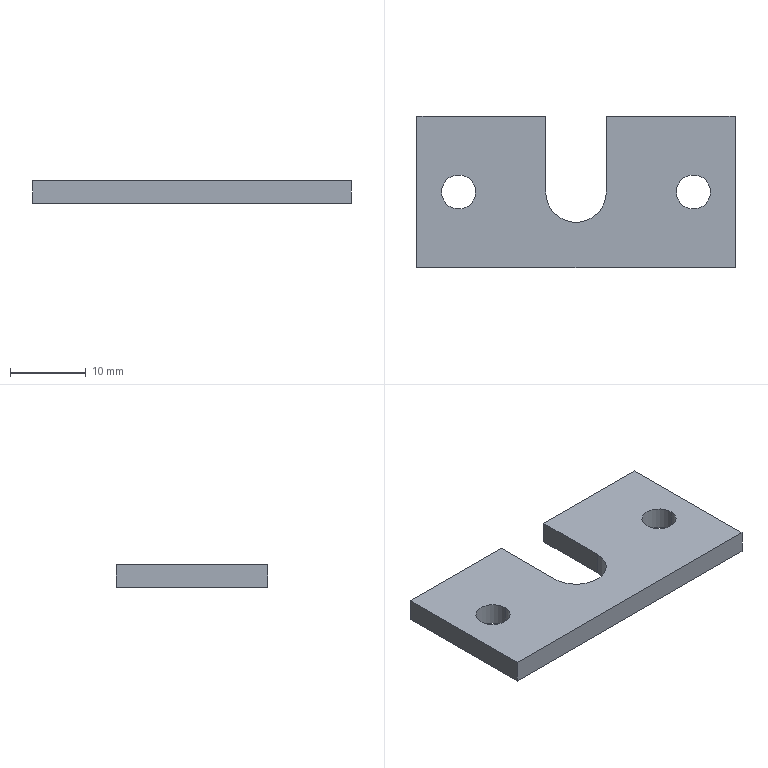Part | SolidWorks | features BaseBody 1 | 1 solid | 14 faces | box 42 x 20 x 3 mm | volume 2109 mm3 | plane 9 | cylinder 5 | commonest cylinder face diameters 4.5 x4 8 x1
STEP:
#1=CARTESIAN_POINT('',(-55.279,98.896,0.));
#2=VERTEX_POINT('',#1);
#3=CARTESIAN_POINT('',(-59.779,98.896,0.));
#4=VERTEX_POINT('',#3);
#5=CARTESIAN_POINT('',(-57.529,98.896,0.));
#6=DIRECTION('',(0.,0.,-1.));
#7=DIRECTION('',(1.,0.,0.));
#8=AXIS2_PLACEMENT_3D('',#5,#6,#7);
#9=CIRCLE('',#8,2.25);
#10=EDGE_CURVE('',#2,#4,#9,.T.);
#11=ORIENTED_EDGE('',*,*,#10,.T.);
#12=CARTESIAN_POINT('',(-59.779,98.896,3.));
#13=VERTEX_POINT('',#12);
#14=CARTESIAN_POINT('',(-59.779,98.896,-43.615));
#15=DIRECTION('',(0.,0.,1.));
#16=VECTOR('',#15,1000.);
#17=LINE('',#14,#16);
#18=EDGE_CURVE('',#4,#13,#17,.T.);
#19=ORIENTED_EDGE('',*,*,#18,.T.);
#20=CARTESIAN_POINT('',(-55.279,98.896,3.));
#21=VERTEX_POINT('',#20);
#22=CARTESIAN_POINT('',(-57.529,98.896,3.));
#23=DIRECTION('',(0.,0.,-1.));
#24=DIRECTION('',(1.,0.,0.));
#25=AXIS2_PLACEMENT_3D('',#22,#23,#24);
#26=CIRCLE('',#25,2.25);
#27=EDGE_CURVE('',#21,#13,#26,.T.);
#28=ORIENTED_EDGE('',*,*,#27,.F.);
#29=CARTESIAN_POINT('',(-55.279,98.896,-43.615));
#30=DIRECTION('',(0.,0.,1.));
#31=VECTOR('',#30,1000.);
#32=LINE('',#29,#31);
#33=EDGE_CURVE('',#2,#21,#32,.T.);
#34=ORIENTED_EDGE('',*,*,#33,.F.);
#35=EDGE_LOOP('',(#11,#19,#28,#34));
#36=FACE_OUTER_BOUND('',#35,.T.);
#37=CARTESIAN_POINT('',(-57.529,98.896,-43.615));
#38=DIRECTION('',(0.,0.,1.));
#39=DIRECTION('',(1.,0.,0.));
#40=AXIS2_PLACEMENT_3D('',#37,#38,#39);
#41=CYLINDRICAL_SURFACE('',#40,2.25);
#42=ADVANCED_FACE('',(#36),#41,.F.);
#43=CARTESIAN_POINT('',(-86.279,98.896,0.));
#44=VERTEX_POINT('',#43);
#45=CARTESIAN_POINT('',(-90.779,98.896,0.));
#46=VERTEX_POINT('',#45);
#47=CARTESIAN_POINT('',(-88.529,98.896,0.));
#48=DIRECTION('',(0.,0.,-1.));
#49=DIRECTION('',(1.,0.,0.));
#50=AXIS2_PLACEMENT_3D('',#47,#48,#49);
#51=CIRCLE('',#50,2.25);
#52=EDGE_CURVE('',#44,#46,#51,.T.);
#53=ORIENTED_EDGE('',*,*,#52,.T.);
#54=CARTESIAN_POINT('',(-90.779,98.896,3.));
#55=VERTEX_POINT('',#54);
#56=CARTESIAN_POINT('',(-90.779,98.896,-43.615));
#57=DIRECTION('',(0.,0.,1.));
#58=VECTOR('',#57,1000.);
#59=LINE('',#56,#58);
#60=EDGE_CURVE('',#46,#55,#59,.T.);
#61=ORIENTED_EDGE('',*,*,#60,.T.);
#62=CARTESIAN_POINT('',(-86.279,98.896,3.));
#63=VERTEX_POINT('',#62);
#64=CARTESIAN_POINT('',(-88.529,98.896,3.));
#65=DIRECTION('',(0.,0.,-1.));
#66=DIRECTION('',(1.,0.,0.));
#67=AXIS2_PLACEMENT_3D('',#64,#65,#66);
#68=CIRCLE('',#67,2.25);
#69=EDGE_CURVE('',#63,#55,#68,.T.);
#70=ORIENTED_EDGE('',*,*,#69,.F.);
#71=CARTESIAN_POINT('',(-86.279,98.896,-43.615));
#72=DIRECTION('',(0.,0.,1.));
#73=VECTOR('',#72,1000.);
#74=LINE('',#71,#73);
#75=EDGE_CURVE('',#44,#63,#74,.T.);
#76=ORIENTED_EDGE('',*,*,#75,.F.);
#77=EDGE_LOOP('',(#53,#61,#70,#76));
#78=FACE_OUTER_BOUND('',#77,.T.);
#79=CARTESIAN_POINT('',(-88.529,98.896,-43.615));
#80=DIRECTION('',(0.,0.,1.));
#81=DIRECTION('',(1.,0.,0.));
#82=AXIS2_PLACEMENT_3D('',#79,#80,#81);
#83=CYLINDRICAL_SURFACE('',#82,2.25);
#84=ADVANCED_FACE('',(#78),#83,.F.);
#85=ORIENTED_EDGE('',*,*,#10,.F.);
#86=CARTESIAN_POINT('',(-57.529,98.896,0.));
#87=DIRECTION('',(0.,0.,-1.));
#88=DIRECTION('',(1.,0.,0.));
#89=AXIS2_PLACEMENT_3D('',#86,#87,#88);
#90=CIRCLE('',#89,2.25);
#91=EDGE_CURVE('',#4,#2,#90,.T.);
#92=ORIENTED_EDGE('',*,*,#91,.F.);
#93=EDGE_LOOP('',(#85,#92));
#94=FACE_BOUND('',#93,.T.);
#95=ORIENTED_EDGE('',*,*,#52,.F.);
#96=CARTESIAN_POINT('',(-88.529,98.896,0.));
#97=DIRECTION('',(0.,0.,-1.));
#98=DIRECTION('',(1.,0.,0.));
#99=AXIS2_PLACEMENT_3D('',#96,#97,#98);
#100=CIRCLE('',#99,2.25);
#101=EDGE_CURVE('',#46,#44,#100,.T.);
#102=ORIENTED_EDGE('',*,*,#101,.F.);
#103=EDGE_LOOP('',(#95,#102));
#104=FACE_BOUND('',#103,.T.);
#105=CARTESIAN_POINT('',(-69.029,98.896,0.));
#106=VERTEX_POINT('',#105);
#107=CARTESIAN_POINT('',(-77.029,98.896,0.));
#108=VERTEX_POINT('',#107);
#109=CARTESIAN_POINT('',(-73.029,98.896,0.));
#110=DIRECTION('',(0.,0.,-1.));
#111=DIRECTION('',(-1.,0.,0.));
#112=AXIS2_PLACEMENT_3D('',#109,#110,#111);
#113=CIRCLE('',#112,4.);
#114=EDGE_CURVE('',#106,#108,#113,.T.);
#115=ORIENTED_EDGE('',*,*,#114,.F.);
#116=CARTESIAN_POINT('',(-69.029,108.896,0.));
#117=VERTEX_POINT('',#116);
#118=CARTESIAN_POINT('',(-69.029,98.896,0.));
#119=DIRECTION('',(0.,-1.,0.));
#120=VECTOR('',#119,1000.);
#121=LINE('',#118,#120);
#122=EDGE_CURVE('',#117,#106,#121,.T.);
#123=ORIENTED_EDGE('',*,*,#122,.F.);
#124=CARTESIAN_POINT('',(-52.029,108.896,0.));
#125=VERTEX_POINT('',#124);
#126=CARTESIAN_POINT('',(-73.029,108.896,0.));
#127=DIRECTION('',(-1.,0.,0.));
#128=VECTOR('',#127,1000.);
#129=LINE('',#126,#128);
#130=EDGE_CURVE('',#125,#117,#129,.T.);
#131=ORIENTED_EDGE('',*,*,#130,.F.);
#132=CARTESIAN_POINT('',(-52.029,88.896,0.));
#133=VERTEX_POINT('',#132);
#134=CARTESIAN_POINT('',(-52.029,98.896,0.));
#135=DIRECTION('',(0.,1.,0.));
#136=VECTOR('',#135,1000.);
#137=LINE('',#134,#136);
#138=EDGE_CURVE('',#133,#125,#137,.T.);
#139=ORIENTED_EDGE('',*,*,#138,.F.);
#140=CARTESIAN_POINT('',(-94.029,88.896,0.));
#141=VERTEX_POINT('',#140);
#142=CARTESIAN_POINT('',(-73.029,88.896,0.));
#143=DIRECTION('',(1.,0.,0.));
#144=VECTOR('',#143,1000.);
#145=LINE('',#142,#144);
#146=EDGE_CURVE('',#141,#133,#145,.T.);
#147=ORIENTED_EDGE('',*,*,#146,.F.);
#148=CARTESIAN_POINT('',(-94.029,108.896,0.));
#149=VERTEX_POINT('',#148);
#150=CARTESIAN_POINT('',(-94.029,98.896,0.));
#151=DIRECTION('',(0.,-1.,0.));
#152=VECTOR('',#151,1000.);
#153=LINE('',#150,#152);
#154=EDGE_CURVE('',#149,#141,#153,.T.);
#155=ORIENTED_EDGE('',*,*,#154,.F.);
#156=CARTESIAN_POINT('',(-77.029,108.896,0.));
#157=VERTEX_POINT('',#156);
#158=CARTESIAN_POINT('',(-73.029,108.896,0.));
#159=DIRECTION('',(-1.,0.,0.));
#160=VECTOR('',#159,1000.);
#161=LINE('',#158,#160);
#162=EDGE_CURVE('',#157,#149,#161,.T.);
#163=ORIENTED_EDGE('',*,*,#162,.F.);
#164=CARTESIAN_POINT('',(-77.029,98.896,0.));
#165=DIRECTION('',(0.,1.,0.));
#166=VECTOR('',#165,1000.);
#167=LINE('',#164,#166);
#168=EDGE_CURVE('',#108,#157,#167,.T.);
#169=ORIENTED_EDGE('',*,*,#168,.F.);
#170=EDGE_LOOP('',(#115,#123,#131,#139,#147,#155,#163,#169));
#171=FACE_OUTER_BOUND('',#170,.T.);
#172=CARTESIAN_POINT('',(-73.029,98.896,0.));
#173=DIRECTION('',(0.,0.,1.));
#174=DIRECTION('',(1.,0.,0.));
#175=AXIS2_PLACEMENT_3D('',#172,#173,#174);
#176=PLANE('',#175);
#177=ADVANCED_FACE('',(#94,#104,#171),#176,.F.);
#178=ORIENTED_EDGE('',*,*,#18,.F.);
#179=ORIENTED_EDGE('',*,*,#91,.T.);
#180=ORIENTED_EDGE('',*,*,#33,.T.);
#181=CARTESIAN_POINT('',(-57.529,98.896,3.));
#182=DIRECTION('',(0.,0.,-1.));
#183=DIRECTION('',(1.,0.,0.));
#184=AXIS2_PLACEMENT_3D('',#181,#182,#183);
#185=CIRCLE('',#184,2.25);
#186=EDGE_CURVE('',#13,#21,#185,.T.);
#187=ORIENTED_EDGE('',*,*,#186,.F.);
#188=EDGE_LOOP('',(#178,#179,#180,#187));
#189=FACE_OUTER_BOUND('',#188,.T.);
#190=CARTESIAN_POINT('',(-57.529,98.896,-43.615));
#191=DIRECTION('',(0.,0.,1.));
#192=DIRECTION('',(1.,0.,0.));
#193=AXIS2_PLACEMENT_3D('',#190,#191,#192);
#194=CYLINDRICAL_SURFACE('',#193,2.25);
#195=ADVANCED_FACE('',(#189),#194,.F.);
#196=ORIENTED_EDGE('',*,*,#60,.F.);
#197=ORIENTED_EDGE('',*,*,#101,.T.);
#198=ORIENTED_EDGE('',*,*,#75,.T.);
#199=CARTESIAN_POINT('',(-88.529,98.896,3.));
#200=DIRECTION('',(0.,0.,-1.));
#201=DIRECTION('',(1.,0.,0.));
#202=AXIS2_PLACEMENT_3D('',#199,#200,#201);
#203=CIRCLE('',#202,2.25);
#204=EDGE_CURVE('',#55,#63,#203,.T.);
#205=ORIENTED_EDGE('',*,*,#204,.F.);
#206=EDGE_LOOP('',(#196,#197,#198,#205));
#207=FACE_OUTER_BOUND('',#206,.T.);
#208=CARTESIAN_POINT('',(-88.529,98.896,-43.615));
#209=DIRECTION('',(0.,0.,1.));
#210=DIRECTION('',(1.,0.,0.));
#211=AXIS2_PLACEMENT_3D('',#208,#209,#210);
#212=CYLINDRICAL_SURFACE('',#211,2.25);
#213=ADVANCED_FACE('',(#207),#212,.F.);
#214=CARTESIAN_POINT('',(-77.029,108.896,3.));
#215=VERTEX_POINT('',#214);
#216=CARTESIAN_POINT('',(-77.029,108.896,3.));
#217=DIRECTION('',(0.,0.,-1.));
#218=VECTOR('',#217,1000.);
#219=LINE('',#216,#218);
#220=EDGE_CURVE('',#215,#157,#219,.T.);
#221=ORIENTED_EDGE('',*,*,#220,.F.);
#222=CARTESIAN_POINT('',(-77.029,98.896,3.));
#223=VERTEX_POINT('',#222);
#224=CARTESIAN_POINT('',(-77.029,108.896,3.));
#225=DIRECTION('',(0.,1.,0.));
#226=VECTOR('',#225,1000.);
#227=LINE('',#224,#226);
#228=EDGE_CURVE('',#223,#215,#227,.T.);
#229=ORIENTED_EDGE('',*,*,#228,.F.);
#230=CARTESIAN_POINT('',(-77.029,98.896,3.));
#231=DIRECTION('',(0.,0.,1.));
#232=VECTOR('',#231,1000.);
#233=LINE('',#230,#232);
#234=EDGE_CURVE('',#108,#223,#233,.T.);
#235=ORIENTED_EDGE('',*,*,#234,.F.);
#236=ORIENTED_EDGE('',*,*,#168,.T.);
#237=EDGE_LOOP('',(#221,#229,#235,#236));
#238=FACE_OUTER_BOUND('',#237,.T.);
#239=CARTESIAN_POINT('',(-77.029,108.896,3.));
#240=DIRECTION('',(-1.,0.,0.));
#241=DIRECTION('',(0.,0.,1.));
#242=AXIS2_PLACEMENT_3D('',#239,#240,#241);
#243=PLANE('',#242);
#244=ADVANCED_FACE('',(#238),#243,.F.);
#245=ORIENTED_EDGE('',*,*,#234,.T.);
#246=CARTESIAN_POINT('',(-69.029,98.896,3.));
#247=VERTEX_POINT('',#246);
#248=CARTESIAN_POINT('',(-73.029,98.896,3.));
#249=DIRECTION('',(0.,0.,-1.));
#250=DIRECTION('',(-1.,0.,0.));
#251=AXIS2_PLACEMENT_3D('',#248,#249,#250);
#252=CIRCLE('',#251,4.);
#253=EDGE_CURVE('',#247,#223,#252,.T.);
#254=ORIENTED_EDGE('',*,*,#253,.F.);
#255=CARTESIAN_POINT('',(-69.029,98.896,3.));
#256=DIRECTION('',(0.,0.,1.));
#257=VECTOR('',#256,1000.);
#258=LINE('',#255,#257);
#259=EDGE_CURVE('',#106,#247,#258,.T.);
#260=ORIENTED_EDGE('',*,*,#259,.F.);
#261=ORIENTED_EDGE('',*,*,#114,.T.);
#262=EDGE_LOOP('',(#245,#254,#260,#261));
#263=FACE_OUTER_BOUND('',#262,.T.);
#264=CARTESIAN_POINT('',(-73.029,98.896,3.));
#265=DIRECTION('',(0.,0.,-1.));
#266=DIRECTION('',(-1.,0.,0.));
#267=AXIS2_PLACEMENT_3D('',#264,#265,#266);
#268=CYLINDRICAL_SURFACE('',#267,4.);
#269=ADVANCED_FACE('',(#263),#268,.F.);
#270=ORIENTED_EDGE('',*,*,#259,.T.);
#271=CARTESIAN_POINT('',(-69.029,108.896,3.));
#272=VERTEX_POINT('',#271);
#273=CARTESIAN_POINT('',(-69.029,98.896,3.));
#274=DIRECTION('',(0.,-1.,0.));
#275=VECTOR('',#274,1000.);
#276=LINE('',#273,#275);
#277=EDGE_CURVE('',#272,#247,#276,.T.);
#278=ORIENTED_EDGE('',*,*,#277,.F.);
#279=CARTESIAN_POINT('',(-69.029,108.896,3.));
#280=DIRECTION('',(0.,0.,1.));
#281=VECTOR('',#280,1000.);
#282=LINE('',#279,#281);
#283=EDGE_CURVE('',#117,#272,#282,.T.);
#284=ORIENTED_EDGE('',*,*,#283,.F.);
#285=ORIENTED_EDGE('',*,*,#122,.T.);
#286=EDGE_LOOP('',(#270,#278,#284,#285));
#287=FACE_OUTER_BOUND('',#286,.T.);
#288=CARTESIAN_POINT('',(-69.029,98.896,3.));
#289=DIRECTION('',(1.,0.,0.));
#290=DIRECTION('',(0.,0.,-1.));
#291=AXIS2_PLACEMENT_3D('',#288,#289,#290);
#292=PLANE('',#291);
#293=ADVANCED_FACE('',(#287),#292,.F.);
#294=CARTESIAN_POINT('',(-52.029,108.896,3.));
#295=VERTEX_POINT('',#294);
#296=CARTESIAN_POINT('',(-52.029,108.896,0.));
#297=DIRECTION('',(0.,0.,-1.));
#298=VECTOR('',#297,1000.);
#299=LINE('',#296,#298);
#300=EDGE_CURVE('',#295,#125,#299,.T.);
#301=ORIENTED_EDGE('',*,*,#300,.T.);
#302=ORIENTED_EDGE('',*,*,#130,.T.);
#303=ORIENTED_EDGE('',*,*,#283,.T.);
#304=CARTESIAN_POINT('',(-94.029,108.896,3.));
#305=DIRECTION('',(1.,0.,0.));
#306=VECTOR('',#305,1000.);
#307=LINE('',#304,#306);
#308=EDGE_CURVE('',#272,#295,#307,.T.);
#309=ORIENTED_EDGE('',*,*,#308,.T.);
#310=EDGE_LOOP('',(#301,#302,#303,#309));
#311=FACE_OUTER_BOUND('',#310,.T.);
#312=CARTESIAN_POINT('',(-94.029,108.896,0.));
#313=DIRECTION('',(0.,1.,0.));
#314=DIRECTION('',(0.,0.,1.));
#315=AXIS2_PLACEMENT_3D('',#312,#313,#314);
#316=PLANE('',#315);
#317=ADVANCED_FACE('',(#311),#316,.T.);
#318=ORIENTED_EDGE('',*,*,#138,.T.);
#319=ORIENTED_EDGE('',*,*,#300,.F.);
#320=CARTESIAN_POINT('',(-52.029,88.896,3.));
#321=VERTEX_POINT('',#320);
#322=CARTESIAN_POINT('',(-52.029,108.896,3.));
#323=DIRECTION('',(0.,-1.,0.));
#324=VECTOR('',#323,1000.);
#325=LINE('',#322,#324);
#326=EDGE_CURVE('',#295,#321,#325,.T.);
#327=ORIENTED_EDGE('',*,*,#326,.T.);
#328=CARTESIAN_POINT('',(-52.029,88.896,0.));
#329=DIRECTION('',(0.,0.,-1.));
#330=VECTOR('',#329,1000.);
#331=LINE('',#328,#330);
#332=EDGE_CURVE('',#321,#133,#331,.T.);
#333=ORIENTED_EDGE('',*,*,#332,.T.);
#334=EDGE_LOOP('',(#318,#319,#327,#333));
#335=FACE_OUTER_BOUND('',#334,.T.);
#336=CARTESIAN_POINT('',(-52.029,108.896,0.));
#337=DIRECTION('',(1.,0.,0.));
#338=DIRECTION('',(0.,0.,-1.));
#339=AXIS2_PLACEMENT_3D('',#336,#337,#338);
#340=PLANE('',#339);
#341=ADVANCED_FACE('',(#335),#340,.T.);
#342=ORIENTED_EDGE('',*,*,#146,.T.);
#343=ORIENTED_EDGE('',*,*,#332,.F.);
#344=CARTESIAN_POINT('',(-94.029,88.896,3.));
#345=VERTEX_POINT('',#344);
#346=CARTESIAN_POINT('',(-52.029,88.896,3.));
#347=DIRECTION('',(-1.,0.,0.));
#348=VECTOR('',#347,1000.);
#349=LINE('',#346,#348);
#350=EDGE_CURVE('',#321,#345,#349,.T.);
#351=ORIENTED_EDGE('',*,*,#350,.T.);
#352=CARTESIAN_POINT('',(-94.029,88.896,0.));
#353=DIRECTION('',(0.,0.,-1.));
#354=VECTOR('',#353,1000.);
#355=LINE('',#352,#354);
#356=EDGE_CURVE('',#345,#141,#355,.T.);
#357=ORIENTED_EDGE('',*,*,#356,.T.);
#358=EDGE_LOOP('',(#342,#343,#351,#357));
#359=FACE_OUTER_BOUND('',#358,.T.);
#360=CARTESIAN_POINT('',(-52.029,88.896,0.));
#361=DIRECTION('',(0.,-1.,0.));
#362=DIRECTION('',(0.,0.,-1.));
#363=AXIS2_PLACEMENT_3D('',#360,#361,#362);
#364=PLANE('',#363);
#365=ADVANCED_FACE('',(#359),#364,.T.);
#366=ORIENTED_EDGE('',*,*,#154,.T.);
#367=ORIENTED_EDGE('',*,*,#356,.F.);
#368=CARTESIAN_POINT('',(-94.029,108.896,3.));
#369=VERTEX_POINT('',#368);
#370=CARTESIAN_POINT('',(-94.029,88.896,3.));
#371=DIRECTION('',(0.,1.,0.));
#372=VECTOR('',#371,1000.);
#373=LINE('',#370,#372);
#374=EDGE_CURVE('',#345,#369,#373,.T.);
#375=ORIENTED_EDGE('',*,*,#374,.T.);
#376=CARTESIAN_POINT('',(-94.029,108.896,0.));
#377=DIRECTION('',(0.,0.,-1.));
#378=VECTOR('',#377,1000.);
#379=LINE('',#376,#378);
#380=EDGE_CURVE('',#369,#149,#379,.T.);
#381=ORIENTED_EDGE('',*,*,#380,.T.);
#382=EDGE_LOOP('',(#366,#367,#375,#381));
#383=FACE_OUTER_BOUND('',#382,.T.);
#384=CARTESIAN_POINT('',(-94.029,88.896,0.));
#385=DIRECTION('',(-1.,0.,0.));
#386=DIRECTION('',(0.,0.,1.));
#387=AXIS2_PLACEMENT_3D('',#384,#385,#386);
#388=PLANE('',#387);
#389=ADVANCED_FACE('',(#383),#388,.T.);
#390=ORIENTED_EDGE('',*,*,#380,.F.);
#391=CARTESIAN_POINT('',(-94.029,108.896,3.));
#392=DIRECTION('',(1.,0.,0.));
#393=VECTOR('',#392,1000.);
#394=LINE('',#391,#393);
#395=EDGE_CURVE('',#369,#215,#394,.T.);
#396=ORIENTED_EDGE('',*,*,#395,.T.);
#397=ORIENTED_EDGE('',*,*,#220,.T.);
#398=ORIENTED_EDGE('',*,*,#162,.T.);
#399=EDGE_LOOP('',(#390,#396,#397,#398));
#400=FACE_OUTER_BOUND('',#399,.T.);
#401=CARTESIAN_POINT('',(-94.029,108.896,0.));
#402=DIRECTION('',(0.,1.,0.));
#403=DIRECTION('',(0.,0.,1.));
#404=AXIS2_PLACEMENT_3D('',#401,#402,#403);
#405=PLANE('',#404);
#406=ADVANCED_FACE('',(#400),#405,.T.);
#407=ORIENTED_EDGE('',*,*,#69,.T.);
#408=ORIENTED_EDGE('',*,*,#204,.T.);
#409=EDGE_LOOP('',(#407,#408));
#410=FACE_BOUND('',#409,.T.);
#411=ORIENTED_EDGE('',*,*,#27,.T.);
#412=ORIENTED_EDGE('',*,*,#186,.T.);
#413=EDGE_LOOP('',(#411,#412));
#414=FACE_BOUND('',#413,.T.);
#415=ORIENTED_EDGE('',*,*,#277,.T.);
#416=ORIENTED_EDGE('',*,*,#253,.T.);
#417=ORIENTED_EDGE('',*,*,#228,.T.);
#418=ORIENTED_EDGE('',*,*,#395,.F.);
#419=ORIENTED_EDGE('',*,*,#374,.F.);
#420=ORIENTED_EDGE('',*,*,#350,.F.);
#421=ORIENTED_EDGE('',*,*,#326,.F.);
#422=ORIENTED_EDGE('',*,*,#308,.F.);
#423=EDGE_LOOP('',(#415,#416,#417,#418,#419,#420,#421,#422));
#424=FACE_OUTER_BOUND('',#423,.T.);
#425=CARTESIAN_POINT('',(-73.029,98.896,3.));
#426=DIRECTION('',(0.,0.,1.));
#427=DIRECTION('',(1.,0.,0.));
#428=AXIS2_PLACEMENT_3D('',#425,#426,#427);
#429=PLANE('',#428);
#430=ADVANCED_FACE('',(#410,#414,#424),#429,.T.);
#431=CLOSED_SHELL('',(#42,#84,#177,#195,#213,#244,#269,#293,#317,#341,#365,#389,#406,#430));
#432=MANIFOLD_SOLID_BREP('',#431);
#433=CARTESIAN_POINT('',(0.,0.,0.));
#434=DIRECTION('',(0.,0.,1.));
#435=DIRECTION('',(1.,0.,0.));
#436=AXIS2_PLACEMENT_3D('',#433,#434,#435);
#437=(LENGTH_UNIT()NAMED_UNIT(*)SI_UNIT(.MILLI.,.METRE.));
#438=UNCERTAINTY_MEASURE_WITH_UNIT(LENGTH_MEASURE(0.00001),#437,'','');
#439=(NAMED_UNIT(*)PLANE_ANGLE_UNIT()SI_UNIT($,.RADIAN.));
#440=(NAMED_UNIT(*)SI_UNIT($,.STERADIAN.)SOLID_ANGLE_UNIT());
#441=(GEOMETRIC_REPRESENTATION_CONTEXT(3)GLOBAL_UNCERTAINTY_ASSIGNED_CONTEXT((#438))GLOBAL_UNIT_ASSIGNED_CONTEXT((#437,#439,#440))REPRESENTATION_CONTEXT('',''));
#442=ADVANCED_BREP_SHAPE_REPRESENTATION('',(#432,#436),#441);